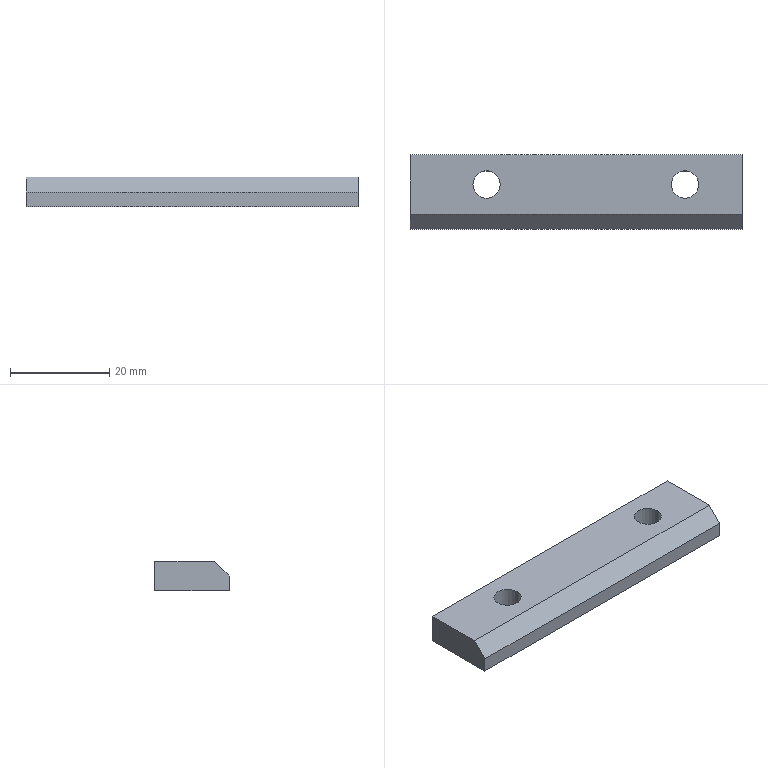Part | STEP file | cover plate | 1 solid | 11 faces | box 66.95 x 15 x 6 mm | volume 5439 mm3 | plane 7 | cylinder 4 | commonest cylinder face diameters 5.5 x4
STEP:
#1=CARTESIAN_POINT('',(0.,0.,0.));
#2=DIRECTION('',(0.,0.,1.));
#3=DIRECTION('',(1.,0.,0.));
#4=AXIS2_PLACEMENT_3D('',#1,#2,#3);
#5=CARTESIAN_POINT('',(-7.25,3.875,0.));
#6=VERTEX_POINT('',#5);
#7=CARTESIAN_POINT('',(-7.25,3.875,6.));
#8=VERTEX_POINT('',#7);
#9=CARTESIAN_POINT('',(-7.25,3.875,6.));
#10=DIRECTION('',(0.,0.,1.));
#11=VECTOR('',#10,1.);
#12=LINE('',#9,#11);
#13=CARTESIAN_POINT('',(-10.,3.875,6.));
#14=DIRECTION('',(0.,0.,1.));
#15=DIRECTION('',(1.,0.,0.));
#16=AXIS2_PLACEMENT_3D('',#13,#14,#15);
#17=CYLINDRICAL_SURFACE('',#16,2.75);
#18=CARTESIAN_POINT('',(6.283,0.));
#19=DIRECTION('',(0.,1.));
#20=VECTOR('',#19,1.);
#21=LINE('',#18,#20);
#22=(GEOMETRIC_REPRESENTATION_CONTEXT(2)PARAMETRIC_REPRESENTATION_CONTEXT()REPRESENTATION_CONTEXT('',''));
#23=DEFINITIONAL_REPRESENTATION('',(#21),#22);
#24=PCURVE('',#17,#23);
#25=CARTESIAN_POINT('',(-10.,3.875,6.));
#26=DIRECTION('',(0.,0.,1.));
#27=DIRECTION('',(1.,0.,0.));
#28=AXIS2_PLACEMENT_3D('',#25,#26,#27);
#29=CYLINDRICAL_SURFACE('',#28,2.75);
#30=CARTESIAN_POINT('',(0.,0.));
#31=DIRECTION('',(0.,1.));
#32=VECTOR('',#31,1.);
#33=LINE('',#30,#32);
#34=(GEOMETRIC_REPRESENTATION_CONTEXT(2)PARAMETRIC_REPRESENTATION_CONTEXT()REPRESENTATION_CONTEXT('',''));
#35=DEFINITIONAL_REPRESENTATION('',(#33),#34);
#36=PCURVE('',#29,#35);
#37=SURFACE_CURVE('',#12,(#24,#36),.PCURVE_S1.);
#38=EDGE_CURVE('',#6,#8,#37,.T.);
#39=ORIENTED_EDGE('',*,*,#38,.T.);
#40=CARTESIAN_POINT('',(-12.75,3.875,6.));
#41=VERTEX_POINT('',#40);
#42=CARTESIAN_POINT('',(-10.,3.875,6.));
#43=DIRECTION('',(0.,0.,1.));
#44=DIRECTION('',(1.,0.,0.));
#45=AXIS2_PLACEMENT_3D('',#42,#43,#44);
#46=CIRCLE('',#45,2.75);
#47=CARTESIAN_POINT('',(0.,0.));
#48=DIRECTION('',(1.,0.));
#49=VECTOR('',#48,1.);
#50=LINE('',#47,#49);
#51=(GEOMETRIC_REPRESENTATION_CONTEXT(2)PARAMETRIC_REPRESENTATION_CONTEXT()REPRESENTATION_CONTEXT('',''));
#52=DEFINITIONAL_REPRESENTATION('',(#50),#51);
#53=PCURVE('',#17,#52);
#54=CARTESIAN_POINT('',(-65.45,-5.125,6.));
#55=DIRECTION('',(0.,0.,1.));
#56=DIRECTION('',(1.,0.,0.));
#57=AXIS2_PLACEMENT_3D('',#54,#55,#56);
#58=PLANE('',#57);
#59=CARTESIAN_POINT('',(55.45,9.));
#60=DIRECTION('',(1.,0.));
#61=AXIS2_PLACEMENT_2D('',#59,#60);
#62=CIRCLE('',#61,2.75);
#63=(GEOMETRIC_REPRESENTATION_CONTEXT(2)PARAMETRIC_REPRESENTATION_CONTEXT()REPRESENTATION_CONTEXT('',''));
#64=DEFINITIONAL_REPRESENTATION('',(#62),#63);
#65=PCURVE('',#58,#64);
#66=SURFACE_CURVE('',#46,(#53,#65),.PCURVE_S1.);
#67=EDGE_CURVE('',#41,#8,#66,.T.);
#68=ORIENTED_EDGE('',*,*,#67,.F.);
#69=CARTESIAN_POINT('',(-12.75,3.875,0.));
#70=VERTEX_POINT('',#69);
#71=CARTESIAN_POINT('',(-12.75,3.875,6.));
#72=DIRECTION('',(0.,0.,1.));
#73=VECTOR('',#72,1.);
#74=LINE('',#71,#73);
#75=CARTESIAN_POINT('',(3.142,0.));
#76=DIRECTION('',(0.,1.));
#77=VECTOR('',#76,1.);
#78=LINE('',#75,#77);
#79=(GEOMETRIC_REPRESENTATION_CONTEXT(2)PARAMETRIC_REPRESENTATION_CONTEXT()REPRESENTATION_CONTEXT('',''));
#80=DEFINITIONAL_REPRESENTATION('',(#78),#79);
#81=PCURVE('',#17,#80);
#82=CARTESIAN_POINT('',(3.142,0.));
#83=DIRECTION('',(0.,1.));
#84=VECTOR('',#83,1.);
#85=LINE('',#82,#84);
#86=(GEOMETRIC_REPRESENTATION_CONTEXT(2)PARAMETRIC_REPRESENTATION_CONTEXT()REPRESENTATION_CONTEXT('',''));
#87=DEFINITIONAL_REPRESENTATION('',(#85),#86);
#88=PCURVE('',#29,#87);
#89=SURFACE_CURVE('',#74,(#81,#88),.PCURVE_S1.);
#90=EDGE_CURVE('',#70,#41,#89,.T.);
#91=ORIENTED_EDGE('',*,*,#90,.F.);
#92=CARTESIAN_POINT('',(-10.,3.875,0.));
#93=DIRECTION('',(0.,0.,1.));
#94=DIRECTION('',(1.,0.,0.));
#95=AXIS2_PLACEMENT_3D('',#92,#93,#94);
#96=CIRCLE('',#95,2.75);
#97=CARTESIAN_POINT('',(0.,-6.));
#98=DIRECTION('',(1.,0.));
#99=VECTOR('',#98,1.);
#100=LINE('',#97,#99);
#101=(GEOMETRIC_REPRESENTATION_CONTEXT(2)PARAMETRIC_REPRESENTATION_CONTEXT()REPRESENTATION_CONTEXT('',''));
#102=DEFINITIONAL_REPRESENTATION('',(#100),#101);
#103=PCURVE('',#17,#102);
#104=CARTESIAN_POINT('',(-65.45,-5.125,0.));
#105=DIRECTION('',(0.,0.,1.));
#106=DIRECTION('',(1.,0.,0.));
#107=AXIS2_PLACEMENT_3D('',#104,#105,#106);
#108=PLANE('',#107);
#109=CARTESIAN_POINT('',(55.45,9.));
#110=DIRECTION('',(1.,0.));
#111=AXIS2_PLACEMENT_2D('',#109,#110);
#112=CIRCLE('',#111,2.75);
#113=(GEOMETRIC_REPRESENTATION_CONTEXT(2)PARAMETRIC_REPRESENTATION_CONTEXT()REPRESENTATION_CONTEXT('',''));
#114=DEFINITIONAL_REPRESENTATION('',(#112),#113);
#115=PCURVE('',#108,#114);
#116=SURFACE_CURVE('',#96,(#103,#115),.PCURVE_S1.);
#117=EDGE_CURVE('',#70,#6,#116,.T.);
#118=ORIENTED_EDGE('',*,*,#117,.T.);
#119=EDGE_LOOP('',(#39,#68,#91,#118));
#120=FACE_BOUND('',#119,.F.);
#121=ADVANCED_FACE('',(#120),#17,.F.);
#122=CARTESIAN_POINT('',(-47.25,3.875,0.));
#123=VERTEX_POINT('',#122);
#124=CARTESIAN_POINT('',(-47.25,3.875,6.));
#125=VERTEX_POINT('',#124);
#126=CARTESIAN_POINT('',(-47.25,3.875,6.));
#127=DIRECTION('',(0.,0.,1.));
#128=VECTOR('',#127,1.);
#129=LINE('',#126,#128);
#130=CARTESIAN_POINT('',(-50.,3.875,6.));
#131=DIRECTION('',(0.,0.,1.));
#132=DIRECTION('',(1.,0.,0.));
#133=AXIS2_PLACEMENT_3D('',#130,#131,#132);
#134=CYLINDRICAL_SURFACE('',#133,2.75);
#135=CARTESIAN_POINT('',(6.283,0.));
#136=DIRECTION('',(0.,1.));
#137=VECTOR('',#136,1.);
#138=LINE('',#135,#137);
#139=(GEOMETRIC_REPRESENTATION_CONTEXT(2)PARAMETRIC_REPRESENTATION_CONTEXT()REPRESENTATION_CONTEXT('',''));
#140=DEFINITIONAL_REPRESENTATION('',(#138),#139);
#141=PCURVE('',#134,#140);
#142=CARTESIAN_POINT('',(-50.,3.875,6.));
#143=DIRECTION('',(0.,0.,1.));
#144=DIRECTION('',(1.,0.,0.));
#145=AXIS2_PLACEMENT_3D('',#142,#143,#144);
#146=CYLINDRICAL_SURFACE('',#145,2.75);
#147=CARTESIAN_POINT('',(0.,0.));
#148=DIRECTION('',(0.,1.));
#149=VECTOR('',#148,1.);
#150=LINE('',#147,#149);
#151=(GEOMETRIC_REPRESENTATION_CONTEXT(2)PARAMETRIC_REPRESENTATION_CONTEXT()REPRESENTATION_CONTEXT('',''));
#152=DEFINITIONAL_REPRESENTATION('',(#150),#151);
#153=PCURVE('',#146,#152);
#154=SURFACE_CURVE('',#129,(#141,#153),.PCURVE_S1.);
#155=EDGE_CURVE('',#123,#125,#154,.T.);
#156=ORIENTED_EDGE('',*,*,#155,.T.);
#157=CARTESIAN_POINT('',(-52.75,3.875,6.));
#158=VERTEX_POINT('',#157);
#159=CARTESIAN_POINT('',(-50.,3.875,6.));
#160=DIRECTION('',(0.,0.,1.));
#161=DIRECTION('',(1.,0.,0.));
#162=AXIS2_PLACEMENT_3D('',#159,#160,#161);
#163=CIRCLE('',#162,2.75);
#164=CARTESIAN_POINT('',(0.,0.));
#165=DIRECTION('',(1.,0.));
#166=VECTOR('',#165,1.);
#167=LINE('',#164,#166);
#168=(GEOMETRIC_REPRESENTATION_CONTEXT(2)PARAMETRIC_REPRESENTATION_CONTEXT()REPRESENTATION_CONTEXT('',''));
#169=DEFINITIONAL_REPRESENTATION('',(#167),#168);
#170=PCURVE('',#134,#169);
#171=CARTESIAN_POINT('',(15.45,9.));
#172=DIRECTION('',(1.,0.));
#173=AXIS2_PLACEMENT_2D('',#171,#172);
#174=CIRCLE('',#173,2.75);
#175=(GEOMETRIC_REPRESENTATION_CONTEXT(2)PARAMETRIC_REPRESENTATION_CONTEXT()REPRESENTATION_CONTEXT('',''));
#176=DEFINITIONAL_REPRESENTATION('',(#174),#175);
#177=PCURVE('',#58,#176);
#178=SURFACE_CURVE('',#163,(#170,#177),.PCURVE_S1.);
#179=EDGE_CURVE('',#158,#125,#178,.T.);
#180=ORIENTED_EDGE('',*,*,#179,.F.);
#181=CARTESIAN_POINT('',(-52.75,3.875,0.));
#182=VERTEX_POINT('',#181);
#183=CARTESIAN_POINT('',(-52.75,3.875,6.));
#184=DIRECTION('',(0.,0.,1.));
#185=VECTOR('',#184,1.);
#186=LINE('',#183,#185);
#187=CARTESIAN_POINT('',(3.142,0.));
#188=DIRECTION('',(0.,1.));
#189=VECTOR('',#188,1.);
#190=LINE('',#187,#189);
#191=(GEOMETRIC_REPRESENTATION_CONTEXT(2)PARAMETRIC_REPRESENTATION_CONTEXT()REPRESENTATION_CONTEXT('',''));
#192=DEFINITIONAL_REPRESENTATION('',(#190),#191);
#193=PCURVE('',#134,#192);
#194=CARTESIAN_POINT('',(3.142,0.));
#195=DIRECTION('',(0.,1.));
#196=VECTOR('',#195,1.);
#197=LINE('',#194,#196);
#198=(GEOMETRIC_REPRESENTATION_CONTEXT(2)PARAMETRIC_REPRESENTATION_CONTEXT()REPRESENTATION_CONTEXT('',''));
#199=DEFINITIONAL_REPRESENTATION('',(#197),#198);
#200=PCURVE('',#146,#199);
#201=SURFACE_CURVE('',#186,(#193,#200),.PCURVE_S1.);
#202=EDGE_CURVE('',#182,#158,#201,.T.);
#203=ORIENTED_EDGE('',*,*,#202,.F.);
#204=CARTESIAN_POINT('',(-50.,3.875,0.));
#205=DIRECTION('',(0.,0.,1.));
#206=DIRECTION('',(1.,0.,0.));
#207=AXIS2_PLACEMENT_3D('',#204,#205,#206);
#208=CIRCLE('',#207,2.75);
#209=CARTESIAN_POINT('',(0.,-6.));
#210=DIRECTION('',(1.,0.));
#211=VECTOR('',#210,1.);
#212=LINE('',#209,#211);
#213=(GEOMETRIC_REPRESENTATION_CONTEXT(2)PARAMETRIC_REPRESENTATION_CONTEXT()REPRESENTATION_CONTEXT('',''));
#214=DEFINITIONAL_REPRESENTATION('',(#212),#213);
#215=PCURVE('',#134,#214);
#216=CARTESIAN_POINT('',(15.45,9.));
#217=DIRECTION('',(1.,0.));
#218=AXIS2_PLACEMENT_2D('',#216,#217);
#219=CIRCLE('',#218,2.75);
#220=(GEOMETRIC_REPRESENTATION_CONTEXT(2)PARAMETRIC_REPRESENTATION_CONTEXT()REPRESENTATION_CONTEXT('',''));
#221=DEFINITIONAL_REPRESENTATION('',(#219),#220);
#222=PCURVE('',#108,#221);
#223=SURFACE_CURVE('',#208,(#215,#222),.PCURVE_S1.);
#224=EDGE_CURVE('',#182,#123,#223,.T.);
#225=ORIENTED_EDGE('',*,*,#224,.T.);
#226=EDGE_LOOP('',(#156,#180,#203,#225));
#227=FACE_BOUND('',#226,.F.);
#228=ADVANCED_FACE('',(#227),#134,.F.);
#229=CARTESIAN_POINT('',(-65.45,-5.125,3.));
#230=VERTEX_POINT('',#229);
#231=CARTESIAN_POINT('',(-65.45,-5.125,0.));
#232=VERTEX_POINT('',#231);
#233=CARTESIAN_POINT('',(-65.45,-5.125,6.));
#234=DIRECTION('',(0.,0.,-1.));
#235=VECTOR('',#234,1.);
#236=LINE('',#233,#235);
#237=CARTESIAN_POINT('',(-65.45,9.875,6.));
#238=DIRECTION('',(1.,0.,0.));
#239=DIRECTION('',(0.,0.,-1.));
#240=AXIS2_PLACEMENT_3D('',#237,#238,#239);
#241=PLANE('',#240);
#242=CARTESIAN_POINT('',(0.,-15.));
#243=DIRECTION('',(1.,0.));
#244=VECTOR('',#243,1.);
#245=LINE('',#242,#244);
#246=(GEOMETRIC_REPRESENTATION_CONTEXT(2)PARAMETRIC_REPRESENTATION_CONTEXT()REPRESENTATION_CONTEXT('',''));
#247=DEFINITIONAL_REPRESENTATION('',(#245),#246);
#248=PCURVE('',#241,#247);
#249=CARTESIAN_POINT('',(-65.45,-5.125,6.));
#250=DIRECTION('',(0.,1.,0.));
#251=DIRECTION('',(0.,0.,1.));
#252=AXIS2_PLACEMENT_3D('',#249,#250,#251);
#253=PLANE('',#252);
#254=CARTESIAN_POINT('',(0.,0.));
#255=DIRECTION('',(-1.,0.));
#256=VECTOR('',#255,1.);
#257=LINE('',#254,#256);
#258=(GEOMETRIC_REPRESENTATION_CONTEXT(2)PARAMETRIC_REPRESENTATION_CONTEXT()REPRESENTATION_CONTEXT('',''));
#259=DEFINITIONAL_REPRESENTATION('',(#257),#258);
#260=PCURVE('',#253,#259);
#261=SURFACE_CURVE('',#236,(#248,#260),.PCURVE_S1.);
#262=EDGE_CURVE('',#230,#232,#261,.T.);
#263=ORIENTED_EDGE('',*,*,#262,.F.);
#264=CARTESIAN_POINT('',(-65.45,-2.125,6.));
#265=VERTEX_POINT('',#264);
#266=CARTESIAN_POINT('',(-65.45,-2.125,6.));
#267=DIRECTION('',(0.,0.7071,0.7071));
#268=VECTOR('',#267,1.);
#269=LINE('',#266,#268);
#270=CARTESIAN_POINT('',(0.,-12.));
#271=DIRECTION('',(-0.7071,0.7071));
#272=VECTOR('',#271,1.);
#273=LINE('',#270,#272);
#274=(GEOMETRIC_REPRESENTATION_CONTEXT(2)PARAMETRIC_REPRESENTATION_CONTEXT()REPRESENTATION_CONTEXT('',''));
#275=DEFINITIONAL_REPRESENTATION('',(#273),#274);
#276=PCURVE('',#241,#275);
#277=CARTESIAN_POINT('',(-65.45,-2.125,6.));
#278=DIRECTION('',(0.,-0.7071,0.7071));
#279=DIRECTION('',(0.,-0.7071,-0.7071));
#280=AXIS2_PLACEMENT_3D('',#277,#278,#279);
#281=PLANE('',#280);
#282=CARTESIAN_POINT('',(0.,0.));
#283=DIRECTION('',(-1.,0.));
#284=VECTOR('',#283,1.);
#285=LINE('',#282,#284);
#286=(GEOMETRIC_REPRESENTATION_CONTEXT(2)PARAMETRIC_REPRESENTATION_CONTEXT()REPRESENTATION_CONTEXT('',''));
#287=DEFINITIONAL_REPRESENTATION('',(#285),#286);
#288=PCURVE('',#281,#287);
#289=SURFACE_CURVE('',#269,(#276,#288),.PCURVE_S1.);
#290=EDGE_CURVE('',#230,#265,#289,.T.);
#291=ORIENTED_EDGE('',*,*,#290,.T.);
#292=CARTESIAN_POINT('',(-65.45,9.875,6.));
#293=VERTEX_POINT('',#292);
#294=CARTESIAN_POINT('',(-65.45,9.875,6.));
#295=DIRECTION('',(0.,-1.,0.));
#296=VECTOR('',#295,1.);
#297=LINE('',#294,#296);
#298=CARTESIAN_POINT('',(0.,0.));
#299=DIRECTION('',(0.,-1.));
#300=VECTOR('',#299,1.);
#301=LINE('',#298,#300);
#302=(GEOMETRIC_REPRESENTATION_CONTEXT(2)PARAMETRIC_REPRESENTATION_CONTEXT()REPRESENTATION_CONTEXT('',''));
#303=DEFINITIONAL_REPRESENTATION('',(#301),#302);
#304=PCURVE('',#241,#303);
#305=CARTESIAN_POINT('',(0.,15.));
#306=DIRECTION('',(0.,-1.));
#307=VECTOR('',#306,1.);
#308=LINE('',#305,#307);
#309=(GEOMETRIC_REPRESENTATION_CONTEXT(2)PARAMETRIC_REPRESENTATION_CONTEXT()REPRESENTATION_CONTEXT('',''));
#310=DEFINITIONAL_REPRESENTATION('',(#308),#309);
#311=PCURVE('',#58,#310);
#312=SURFACE_CURVE('',#297,(#304,#311),.PCURVE_S1.);
#313=EDGE_CURVE('',#293,#265,#312,.T.);
#314=ORIENTED_EDGE('',*,*,#313,.F.);
#315=CARTESIAN_POINT('',(-65.45,9.875,0.));
#316=VERTEX_POINT('',#315);
#317=CARTESIAN_POINT('',(-65.45,9.875,6.));
#318=DIRECTION('',(0.,0.,-1.));
#319=VECTOR('',#318,1.);
#320=LINE('',#317,#319);
#321=CARTESIAN_POINT('',(0.,0.));
#322=DIRECTION('',(1.,0.));
#323=VECTOR('',#322,1.);
#324=LINE('',#321,#323);
#325=(GEOMETRIC_REPRESENTATION_CONTEXT(2)PARAMETRIC_REPRESENTATION_CONTEXT()REPRESENTATION_CONTEXT('',''));
#326=DEFINITIONAL_REPRESENTATION('',(#324),#325);
#327=PCURVE('',#241,#326);
#328=CARTESIAN_POINT('',(-65.45,9.875,6.));
#329=DIRECTION('',(0.,-1.,0.));
#330=DIRECTION('',(0.,0.,-1.));
#331=AXIS2_PLACEMENT_3D('',#328,#329,#330);
#332=PLANE('',#331);
#333=CARTESIAN_POINT('',(0.,0.));
#334=DIRECTION('',(1.,0.));
#335=VECTOR('',#334,1.);
#336=LINE('',#333,#335);
#337=(GEOMETRIC_REPRESENTATION_CONTEXT(2)PARAMETRIC_REPRESENTATION_CONTEXT()REPRESENTATION_CONTEXT('',''));
#338=DEFINITIONAL_REPRESENTATION('',(#336),#337);
#339=PCURVE('',#332,#338);
#340=SURFACE_CURVE('',#320,(#327,#339),.PCURVE_S1.);
#341=EDGE_CURVE('',#293,#316,#340,.T.);
#342=ORIENTED_EDGE('',*,*,#341,.T.);
#343=CARTESIAN_POINT('',(-65.45,9.875,0.));
#344=DIRECTION('',(0.,-1.,0.));
#345=VECTOR('',#344,1.);
#346=LINE('',#343,#345);
#347=CARTESIAN_POINT('',(6.,0.));
#348=DIRECTION('',(0.,-1.));
#349=VECTOR('',#348,1.);
#350=LINE('',#347,#349);
#351=(GEOMETRIC_REPRESENTATION_CONTEXT(2)PARAMETRIC_REPRESENTATION_CONTEXT()REPRESENTATION_CONTEXT('',''));
#352=DEFINITIONAL_REPRESENTATION('',(#350),#351);
#353=PCURVE('',#241,#352);
#354=CARTESIAN_POINT('',(0.,15.));
#355=DIRECTION('',(0.,-1.));
#356=VECTOR('',#355,1.);
#357=LINE('',#354,#356);
#358=(GEOMETRIC_REPRESENTATION_CONTEXT(2)PARAMETRIC_REPRESENTATION_CONTEXT()REPRESENTATION_CONTEXT('',''));
#359=DEFINITIONAL_REPRESENTATION('',(#357),#358);
#360=PCURVE('',#108,#359);
#361=SURFACE_CURVE('',#346,(#353,#360),.PCURVE_S1.);
#362=EDGE_CURVE('',#316,#232,#361,.T.);
#363=ORIENTED_EDGE('',*,*,#362,.T.);
#364=EDGE_LOOP('',(#263,#291,#314,#342,#363));
#365=FACE_BOUND('',#364,.T.);
#366=ADVANCED_FACE('',(#365),#241,.F.);
#367=CARTESIAN_POINT('',(1.5,-5.125,0.));
#368=VERTEX_POINT('',#367);
#369=CARTESIAN_POINT('',(-65.45,-5.125,0.));
#370=DIRECTION('',(1.,0.,0.));
#371=VECTOR('',#370,1.);
#372=LINE('',#369,#371);
#373=CARTESIAN_POINT('',(-6.,0.));
#374=DIRECTION('',(0.,1.));
#375=VECTOR('',#374,1.);
#376=LINE('',#373,#375);
#377=(GEOMETRIC_REPRESENTATION_CONTEXT(2)PARAMETRIC_REPRESENTATION_CONTEXT()REPRESENTATION_CONTEXT('',''));
#378=DEFINITIONAL_REPRESENTATION('',(#376),#377);
#379=PCURVE('',#253,#378);
#380=CARTESIAN_POINT('',(0.,0.));
#381=DIRECTION('',(1.,0.));
#382=VECTOR('',#381,1.);
#383=LINE('',#380,#382);
#384=(GEOMETRIC_REPRESENTATION_CONTEXT(2)PARAMETRIC_REPRESENTATION_CONTEXT()REPRESENTATION_CONTEXT('',''));
#385=DEFINITIONAL_REPRESENTATION('',(#383),#384);
#386=PCURVE('',#108,#385);
#387=SURFACE_CURVE('',#372,(#379,#386),.PCURVE_S1.);
#388=EDGE_CURVE('',#232,#368,#387,.T.);
#389=ORIENTED_EDGE('',*,*,#388,.T.);
#390=CARTESIAN_POINT('',(1.5,-5.125,3.));
#391=VERTEX_POINT('',#390);
#392=CARTESIAN_POINT('',(1.5,-5.125,3.));
#393=DIRECTION('',(0.,0.,-1.));
#394=VECTOR('',#393,1.);
#395=LINE('',#392,#394);
#396=CARTESIAN_POINT('',(-3.,66.95));
#397=DIRECTION('',(-1.,0.));
#398=VECTOR('',#397,1.);
#399=LINE('',#396,#398);
#400=(GEOMETRIC_REPRESENTATION_CONTEXT(2)PARAMETRIC_REPRESENTATION_CONTEXT()REPRESENTATION_CONTEXT('',''));
#401=DEFINITIONAL_REPRESENTATION('',(#399),#400);
#402=PCURVE('',#253,#401);
#403=CARTESIAN_POINT('',(1.5,9.875,6.));
#404=DIRECTION('',(1.,0.,0.));
#405=DIRECTION('',(0.,0.,-1.));
#406=AXIS2_PLACEMENT_3D('',#403,#404,#405);
#407=PLANE('',#406);
#408=CARTESIAN_POINT('',(3.,-15.));
#409=DIRECTION('',(1.,0.));
#410=VECTOR('',#409,1.);
#411=LINE('',#408,#410);
#412=(GEOMETRIC_REPRESENTATION_CONTEXT(2)PARAMETRIC_REPRESENTATION_CONTEXT()REPRESENTATION_CONTEXT('',''));
#413=DEFINITIONAL_REPRESENTATION('',(#411),#412);
#414=PCURVE('',#407,#413);
#415=SURFACE_CURVE('',#395,(#402,#414),.PCURVE_S1.);
#416=EDGE_CURVE('',#391,#368,#415,.T.);
#417=ORIENTED_EDGE('',*,*,#416,.F.);
#418=CARTESIAN_POINT('',(-65.45,-5.125,3.));
#419=DIRECTION('',(-1.,0.,0.));
#420=VECTOR('',#419,1.);
#421=LINE('',#418,#420);
#422=CARTESIAN_POINT('',(-3.,0.));
#423=DIRECTION('',(0.,-1.));
#424=VECTOR('',#423,1.);
#425=LINE('',#422,#424);
#426=(GEOMETRIC_REPRESENTATION_CONTEXT(2)PARAMETRIC_REPRESENTATION_CONTEXT()REPRESENTATION_CONTEXT('',''));
#427=DEFINITIONAL_REPRESENTATION('',(#425),#426);
#428=PCURVE('',#253,#427);
#429=CARTESIAN_POINT('',(4.243,0.));
#430=DIRECTION('',(0.,-1.));
#431=VECTOR('',#430,1.);
#432=LINE('',#429,#431);
#433=(GEOMETRIC_REPRESENTATION_CONTEXT(2)PARAMETRIC_REPRESENTATION_CONTEXT()REPRESENTATION_CONTEXT('',''));
#434=DEFINITIONAL_REPRESENTATION('',(#432),#433);
#435=PCURVE('',#281,#434);
#436=SURFACE_CURVE('',#421,(#428,#435),.PCURVE_S1.);
#437=EDGE_CURVE('',#391,#230,#436,.T.);
#438=ORIENTED_EDGE('',*,*,#437,.T.);
#439=ORIENTED_EDGE('',*,*,#262,.T.);
#440=EDGE_LOOP('',(#389,#417,#438,#439));
#441=FACE_BOUND('',#440,.T.);
#442=ADVANCED_FACE('',(#441),#253,.F.);
#443=CARTESIAN_POINT('',(1.5,9.875,0.));
#444=VERTEX_POINT('',#443);
#445=CARTESIAN_POINT('',(-65.45,9.875,0.));
#446=DIRECTION('',(-1.,0.,0.));
#447=VECTOR('',#446,1.);
#448=LINE('',#445,#447);
#449=CARTESIAN_POINT('',(6.,0.));
#450=DIRECTION('',(0.,-1.));
#451=VECTOR('',#450,1.);
#452=LINE('',#449,#451);
#453=(GEOMETRIC_REPRESENTATION_CONTEXT(2)PARAMETRIC_REPRESENTATION_CONTEXT()REPRESENTATION_CONTEXT('',''));
#454=DEFINITIONAL_REPRESENTATION('',(#452),#453);
#455=PCURVE('',#332,#454);
#456=CARTESIAN_POINT('',(0.,15.));
#457=DIRECTION('',(-1.,0.));
#458=VECTOR('',#457,1.);
#459=LINE('',#456,#458);
#460=(GEOMETRIC_REPRESENTATION_CONTEXT(2)PARAMETRIC_REPRESENTATION_CONTEXT()REPRESENTATION_CONTEXT('',''));
#461=DEFINITIONAL_REPRESENTATION('',(#459),#460);
#462=PCURVE('',#108,#461);
#463=SURFACE_CURVE('',#448,(#455,#462),.PCURVE_S1.);
#464=EDGE_CURVE('',#444,#316,#463,.T.);
#465=ORIENTED_EDGE('',*,*,#464,.T.);
#466=ORIENTED_EDGE('',*,*,#341,.F.);
#467=CARTESIAN_POINT('',(1.5,9.875,6.));
#468=VERTEX_POINT('',#467);
#469=CARTESIAN_POINT('',(-65.45,9.875,6.));
#470=DIRECTION('',(-1.,0.,0.));
#471=VECTOR('',#470,1.);
#472=LINE('',#469,#471);
#473=CARTESIAN_POINT('',(0.,0.));
#474=DIRECTION('',(0.,-1.));
#475=VECTOR('',#474,1.);
#476=LINE('',#473,#475);
#477=(GEOMETRIC_REPRESENTATION_CONTEXT(2)PARAMETRIC_REPRESENTATION_CONTEXT()REPRESENTATION_CONTEXT('',''));
#478=DEFINITIONAL_REPRESENTATION('',(#476),#477);
#479=PCURVE('',#332,#478);
#480=CARTESIAN_POINT('',(0.,15.));
#481=DIRECTION('',(-1.,0.));
#482=VECTOR('',#481,1.);
#483=LINE('',#480,#482);
#484=(GEOMETRIC_REPRESENTATION_CONTEXT(2)PARAMETRIC_REPRESENTATION_CONTEXT()REPRESENTATION_CONTEXT('',''));
#485=DEFINITIONAL_REPRESENTATION('',(#483),#484);
#486=PCURVE('',#58,#485);
#487=SURFACE_CURVE('',#472,(#479,#486),.PCURVE_S1.);
#488=EDGE_CURVE('',#468,#293,#487,.T.);
#489=ORIENTED_EDGE('',*,*,#488,.F.);
#490=CARTESIAN_POINT('',(1.5,9.875,0.));
#491=DIRECTION('',(0.,0.,1.));
#492=VECTOR('',#491,1.);
#493=LINE('',#490,#492);
#494=CARTESIAN_POINT('',(6.,66.95));
#495=DIRECTION('',(-1.,0.));
#496=VECTOR('',#495,1.);
#497=LINE('',#494,#496);
#498=(GEOMETRIC_REPRESENTATION_CONTEXT(2)PARAMETRIC_REPRESENTATION_CONTEXT()REPRESENTATION_CONTEXT('',''));
#499=DEFINITIONAL_REPRESENTATION('',(#497),#498);
#500=PCURVE('',#332,#499);
#501=CARTESIAN_POINT('',(6.,0.));
#502=DIRECTION('',(-1.,0.));
#503=VECTOR('',#502,1.);
#504=LINE('',#501,#503);
#505=(GEOMETRIC_REPRESENTATION_CONTEXT(2)PARAMETRIC_REPRESENTATION_CONTEXT()REPRESENTATION_CONTEXT('',''));
#506=DEFINITIONAL_REPRESENTATION('',(#504),#505);
#507=PCURVE('',#407,#506);
#508=SURFACE_CURVE('',#493,(#500,#507),.PCURVE_S1.);
#509=EDGE_CURVE('',#444,#468,#508,.T.);
#510=ORIENTED_EDGE('',*,*,#509,.F.);
#511=EDGE_LOOP('',(#465,#466,#489,#510));
#512=FACE_BOUND('',#511,.T.);
#513=ADVANCED_FACE('',(#512),#332,.F.);
#514=CARTESIAN_POINT('',(-10.,3.875,6.));
#515=DIRECTION('',(0.,0.,1.));
#516=DIRECTION('',(1.,0.,0.));
#517=AXIS2_PLACEMENT_3D('',#514,#515,#516);
#518=CIRCLE('',#517,2.75);
#519=CARTESIAN_POINT('',(55.45,9.));
#520=DIRECTION('',(1.,0.));
#521=AXIS2_PLACEMENT_2D('',#519,#520);
#522=CIRCLE('',#521,2.75);
#523=(GEOMETRIC_REPRESENTATION_CONTEXT(2)PARAMETRIC_REPRESENTATION_CONTEXT()REPRESENTATION_CONTEXT('',''));
#524=DEFINITIONAL_REPRESENTATION('',(#522),#523);
#525=PCURVE('',#58,#524);
#526=CARTESIAN_POINT('',(0.,0.));
#527=DIRECTION('',(1.,0.));
#528=VECTOR('',#527,1.);
#529=LINE('',#526,#528);
#530=(GEOMETRIC_REPRESENTATION_CONTEXT(2)PARAMETRIC_REPRESENTATION_CONTEXT()REPRESENTATION_CONTEXT('',''));
#531=DEFINITIONAL_REPRESENTATION('',(#529),#530);
#532=PCURVE('',#29,#531);
#533=SURFACE_CURVE('',#518,(#525,#532),.PCURVE_S1.);
#534=EDGE_CURVE('',#8,#41,#533,.T.);
#535=ORIENTED_EDGE('',*,*,#534,.F.);
#536=ORIENTED_EDGE('',*,*,#67,.F.);
#537=EDGE_LOOP('',(#535,#536));
#538=FACE_BOUND('',#537,.T.);
#539=CARTESIAN_POINT('',(-50.,3.875,6.));
#540=DIRECTION('',(0.,0.,1.));
#541=DIRECTION('',(1.,0.,0.));
#542=AXIS2_PLACEMENT_3D('',#539,#540,#541);
#543=CIRCLE('',#542,2.75);
#544=CARTESIAN_POINT('',(15.45,9.));
#545=DIRECTION('',(1.,0.));
#546=AXIS2_PLACEMENT_2D('',#544,#545);
#547=CIRCLE('',#546,2.75);
#548=(GEOMETRIC_REPRESENTATION_CONTEXT(2)PARAMETRIC_REPRESENTATION_CONTEXT()REPRESENTATION_CONTEXT('',''));
#549=DEFINITIONAL_REPRESENTATION('',(#547),#548);
#550=PCURVE('',#58,#549);
#551=CARTESIAN_POINT('',(0.,0.));
#552=DIRECTION('',(1.,0.));
#553=VECTOR('',#552,1.);
#554=LINE('',#551,#553);
#555=(GEOMETRIC_REPRESENTATION_CONTEXT(2)PARAMETRIC_REPRESENTATION_CONTEXT()REPRESENTATION_CONTEXT('',''));
#556=DEFINITIONAL_REPRESENTATION('',(#554),#555);
#557=PCURVE('',#146,#556);
#558=SURFACE_CURVE('',#543,(#550,#557),.PCURVE_S1.);
#559=EDGE_CURVE('',#125,#158,#558,.T.);
#560=ORIENTED_EDGE('',*,*,#559,.F.);
#561=ORIENTED_EDGE('',*,*,#179,.F.);
#562=EDGE_LOOP('',(#560,#561));
#563=FACE_BOUND('',#562,.T.);
#564=ORIENTED_EDGE('',*,*,#313,.T.);
#565=CARTESIAN_POINT('',(1.5,-2.125,6.));
#566=VERTEX_POINT('',#565);
#567=CARTESIAN_POINT('',(-30.,-2.125,6.));
#568=DIRECTION('',(1.,0.,0.));
#569=VECTOR('',#568,1.);
#570=LINE('',#567,#569);
#571=CARTESIAN_POINT('',(35.45,3.));
#572=DIRECTION('',(1.,0.));
#573=VECTOR('',#572,1.);
#574=LINE('',#571,#573);
#575=(GEOMETRIC_REPRESENTATION_CONTEXT(2)PARAMETRIC_REPRESENTATION_CONTEXT()REPRESENTATION_CONTEXT('',''));
#576=DEFINITIONAL_REPRESENTATION('',(#574),#575);
#577=PCURVE('',#58,#576);
#578=CARTESIAN_POINT('',(0.,35.45));
#579=DIRECTION('',(0.,1.));
#580=VECTOR('',#579,1.);
#581=LINE('',#578,#580);
#582=(GEOMETRIC_REPRESENTATION_CONTEXT(2)PARAMETRIC_REPRESENTATION_CONTEXT()REPRESENTATION_CONTEXT('',''));
#583=DEFINITIONAL_REPRESENTATION('',(#581),#582);
#584=PCURVE('',#281,#583);
#585=SURFACE_CURVE('',#570,(#577,#584),.PCURVE_S1.);
#586=EDGE_CURVE('',#265,#566,#585,.T.);
#587=ORIENTED_EDGE('',*,*,#586,.T.);
#588=CARTESIAN_POINT('',(1.5,9.875,6.));
#589=DIRECTION('',(0.,-1.,0.));
#590=VECTOR('',#589,1.);
#591=LINE('',#588,#590);
#592=CARTESIAN_POINT('',(66.95,15.));
#593=DIRECTION('',(0.,-1.));
#594=VECTOR('',#593,1.);
#595=LINE('',#592,#594);
#596=(GEOMETRIC_REPRESENTATION_CONTEXT(2)PARAMETRIC_REPRESENTATION_CONTEXT()REPRESENTATION_CONTEXT('',''));
#597=DEFINITIONAL_REPRESENTATION('',(#595),#596);
#598=PCURVE('',#58,#597);
#599=CARTESIAN_POINT('',(0.,0.));
#600=DIRECTION('',(0.,-1.));
#601=VECTOR('',#600,1.);
#602=LINE('',#599,#601);
#603=(GEOMETRIC_REPRESENTATION_CONTEXT(2)PARAMETRIC_REPRESENTATION_CONTEXT()REPRESENTATION_CONTEXT('',''));
#604=DEFINITIONAL_REPRESENTATION('',(#602),#603);
#605=PCURVE('',#407,#604);
#606=SURFACE_CURVE('',#591,(#598,#605),.PCURVE_S1.);
#607=EDGE_CURVE('',#468,#566,#606,.T.);
#608=ORIENTED_EDGE('',*,*,#607,.F.);
#609=ORIENTED_EDGE('',*,*,#488,.T.);
#610=EDGE_LOOP('',(#564,#587,#608,#609));
#611=FACE_BOUND('',#610,.T.);
#612=ADVANCED_FACE('',(#538,#563,#611),#58,.T.);
#613=CARTESIAN_POINT('',(-10.,3.875,0.));
#614=DIRECTION('',(0.,0.,1.));
#615=DIRECTION('',(1.,0.,0.));
#616=AXIS2_PLACEMENT_3D('',#613,#614,#615);
#617=CIRCLE('',#616,2.75);
#618=CARTESIAN_POINT('',(55.45,9.));
#619=DIRECTION('',(1.,0.));
#620=AXIS2_PLACEMENT_2D('',#618,#619);
#621=CIRCLE('',#620,2.75);
#622=(GEOMETRIC_REPRESENTATION_CONTEXT(2)PARAMETRIC_REPRESENTATION_CONTEXT()REPRESENTATION_CONTEXT('',''));
#623=DEFINITIONAL_REPRESENTATION('',(#621),#622);
#624=PCURVE('',#108,#623);
#625=CARTESIAN_POINT('',(0.,-6.));
#626=DIRECTION('',(1.,0.));
#627=VECTOR('',#626,1.);
#628=LINE('',#625,#627);
#629=(GEOMETRIC_REPRESENTATION_CONTEXT(2)PARAMETRIC_REPRESENTATION_CONTEXT()REPRESENTATION_CONTEXT('',''));
#630=DEFINITIONAL_REPRESENTATION('',(#628),#629);
#631=PCURVE('',#29,#630);
#632=SURFACE_CURVE('',#617,(#624,#631),.PCURVE_S1.);
#633=EDGE_CURVE('',#6,#70,#632,.T.);
#634=ORIENTED_EDGE('',*,*,#633,.T.);
#635=ORIENTED_EDGE('',*,*,#117,.T.);
#636=EDGE_LOOP('',(#634,#635));
#637=FACE_BOUND('',#636,.T.);
#638=CARTESIAN_POINT('',(-50.,3.875,0.));
#639=DIRECTION('',(0.,0.,1.));
#640=DIRECTION('',(1.,0.,0.));
#641=AXIS2_PLACEMENT_3D('',#638,#639,#640);
#642=CIRCLE('',#641,2.75);
#643=CARTESIAN_POINT('',(15.45,9.));
#644=DIRECTION('',(1.,0.));
#645=AXIS2_PLACEMENT_2D('',#643,#644);
#646=CIRCLE('',#645,2.75);
#647=(GEOMETRIC_REPRESENTATION_CONTEXT(2)PARAMETRIC_REPRESENTATION_CONTEXT()REPRESENTATION_CONTEXT('',''));
#648=DEFINITIONAL_REPRESENTATION('',(#646),#647);
#649=PCURVE('',#108,#648);
#650=CARTESIAN_POINT('',(0.,-6.));
#651=DIRECTION('',(1.,0.));
#652=VECTOR('',#651,1.);
#653=LINE('',#650,#652);
#654=(GEOMETRIC_REPRESENTATION_CONTEXT(2)PARAMETRIC_REPRESENTATION_CONTEXT()REPRESENTATION_CONTEXT('',''));
#655=DEFINITIONAL_REPRESENTATION('',(#653),#654);
#656=PCURVE('',#146,#655);
#657=SURFACE_CURVE('',#642,(#649,#656),.PCURVE_S1.);
#658=EDGE_CURVE('',#123,#182,#657,.T.);
#659=ORIENTED_EDGE('',*,*,#658,.T.);
#660=ORIENTED_EDGE('',*,*,#224,.T.);
#661=EDGE_LOOP('',(#659,#660));
#662=FACE_BOUND('',#661,.T.);
#663=ORIENTED_EDGE('',*,*,#362,.F.);
#664=ORIENTED_EDGE('',*,*,#464,.F.);
#665=CARTESIAN_POINT('',(1.5,-5.125,0.));
#666=DIRECTION('',(0.,1.,0.));
#667=VECTOR('',#666,1.);
#668=LINE('',#665,#667);
#669=CARTESIAN_POINT('',(66.95,0.));
#670=DIRECTION('',(0.,1.));
#671=VECTOR('',#670,1.);
#672=LINE('',#669,#671);
#673=(GEOMETRIC_REPRESENTATION_CONTEXT(2)PARAMETRIC_REPRESENTATION_CONTEXT()REPRESENTATION_CONTEXT('',''));
#674=DEFINITIONAL_REPRESENTATION('',(#672),#673);
#675=PCURVE('',#108,#674);
#676=CARTESIAN_POINT('',(6.,-15.));
#677=DIRECTION('',(0.,1.));
#678=VECTOR('',#677,1.);
#679=LINE('',#676,#678);
#680=(GEOMETRIC_REPRESENTATION_CONTEXT(2)PARAMETRIC_REPRESENTATION_CONTEXT()REPRESENTATION_CONTEXT('',''));
#681=DEFINITIONAL_REPRESENTATION('',(#679),#680);
#682=PCURVE('',#407,#681);
#683=SURFACE_CURVE('',#668,(#675,#682),.PCURVE_S1.);
#684=EDGE_CURVE('',#368,#444,#683,.T.);
#685=ORIENTED_EDGE('',*,*,#684,.F.);
#686=ORIENTED_EDGE('',*,*,#388,.F.);
#687=EDGE_LOOP('',(#663,#664,#685,#686));
#688=FACE_BOUND('',#687,.T.);
#689=ADVANCED_FACE('',(#637,#662,#688),#108,.F.);
#690=ORIENTED_EDGE('',*,*,#559,.F.);
#691=ORIENTED_EDGE('',*,*,#155,.F.);
#692=ORIENTED_EDGE('',*,*,#658,.T.);
#693=ORIENTED_EDGE('',*,*,#202,.T.);
#694=EDGE_LOOP('',(#690,#691,#692,#693));
#695=FACE_BOUND('',#694,.F.);
#696=ADVANCED_FACE('',(#695),#146,.F.);
#697=ORIENTED_EDGE('',*,*,#290,.F.);
#698=ORIENTED_EDGE('',*,*,#437,.F.);
#699=CARTESIAN_POINT('',(1.5,-2.125,6.));
#700=DIRECTION('',(0.,-0.7071,-0.7071));
#701=VECTOR('',#700,1.);
#702=LINE('',#699,#701);
#703=CARTESIAN_POINT('',(0.,66.95));
#704=DIRECTION('',(1.,0.));
#705=VECTOR('',#704,1.);
#706=LINE('',#703,#705);
#707=(GEOMETRIC_REPRESENTATION_CONTEXT(2)PARAMETRIC_REPRESENTATION_CONTEXT()REPRESENTATION_CONTEXT('',''));
#708=DEFINITIONAL_REPRESENTATION('',(#706),#707);
#709=PCURVE('',#281,#708);
#710=CARTESIAN_POINT('',(0.,-12.));
#711=DIRECTION('',(0.7071,-0.7071));
#712=VECTOR('',#711,1.);
#713=LINE('',#710,#712);
#714=(GEOMETRIC_REPRESENTATION_CONTEXT(2)PARAMETRIC_REPRESENTATION_CONTEXT()REPRESENTATION_CONTEXT('',''));
#715=DEFINITIONAL_REPRESENTATION('',(#713),#714);
#716=PCURVE('',#407,#715);
#717=SURFACE_CURVE('',#702,(#709,#716),.PCURVE_S1.);
#718=EDGE_CURVE('',#566,#391,#717,.T.);
#719=ORIENTED_EDGE('',*,*,#718,.F.);
#720=ORIENTED_EDGE('',*,*,#586,.F.);
#721=EDGE_LOOP('',(#697,#698,#719,#720));
#722=FACE_BOUND('',#721,.T.);
#723=ADVANCED_FACE('',(#722),#281,.T.);
#724=ORIENTED_EDGE('',*,*,#509,.T.);
#725=ORIENTED_EDGE('',*,*,#607,.T.);
#726=ORIENTED_EDGE('',*,*,#718,.T.);
#727=ORIENTED_EDGE('',*,*,#416,.T.);
#728=ORIENTED_EDGE('',*,*,#684,.T.);
#729=EDGE_LOOP('',(#724,#725,#726,#727,#728));
#730=FACE_BOUND('',#729,.T.);
#731=ADVANCED_FACE('',(#730),#407,.T.);
#732=ORIENTED_EDGE('',*,*,#534,.F.);
#733=ORIENTED_EDGE('',*,*,#38,.F.);
#734=ORIENTED_EDGE('',*,*,#633,.T.);
#735=ORIENTED_EDGE('',*,*,#90,.T.);
#736=EDGE_LOOP('',(#732,#733,#734,#735));
#737=FACE_BOUND('',#736,.F.);
#738=ADVANCED_FACE('',(#737),#29,.F.);
#739=CLOSED_SHELL('',(#121,#228,#366,#442,#513,#612,#689,#696,#723,#731,#738));
#740=MANIFOLD_SOLID_BREP('',#739);
#741=(LENGTH_UNIT()NAMED_UNIT(*)SI_UNIT(.MILLI.,.METRE.));
#742=UNCERTAINTY_MEASURE_WITH_UNIT(LENGTH_MEASURE(0.0000001),#741,'','');
#743=(NAMED_UNIT(*)PLANE_ANGLE_UNIT()SI_UNIT($,.RADIAN.));
#744=(NAMED_UNIT(*)SI_UNIT($,.STERADIAN.)SOLID_ANGLE_UNIT());
#745=(GEOMETRIC_REPRESENTATION_CONTEXT(3)GLOBAL_UNCERTAINTY_ASSIGNED_CONTEXT((#742))GLOBAL_UNIT_ASSIGNED_CONTEXT((#741,#743,#744))REPRESENTATION_CONTEXT('',''));
#746=ADVANCED_BREP_SHAPE_REPRESENTATION('',(#4,#740),#745);